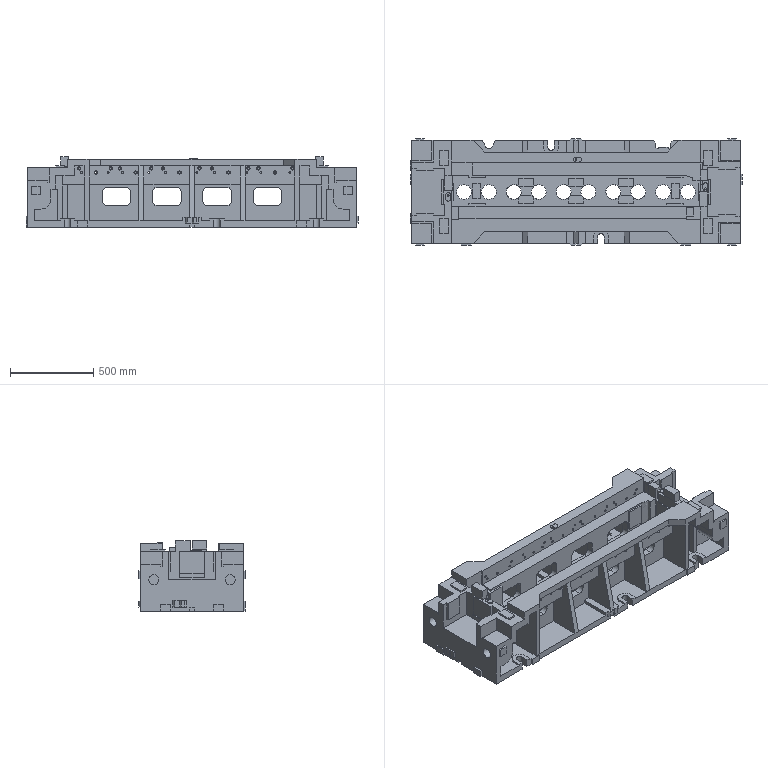Part | NX | features solid 2 | 1 solid | 778 faces | box 2000 x 640 x 425 mm | volume 163390504 mm3 | plane 625 | cylinder 152 | spline 1 | commonest cylinder face diameters 60 x36 13 x30 20 x30 12 x20 90 x16 40 x7